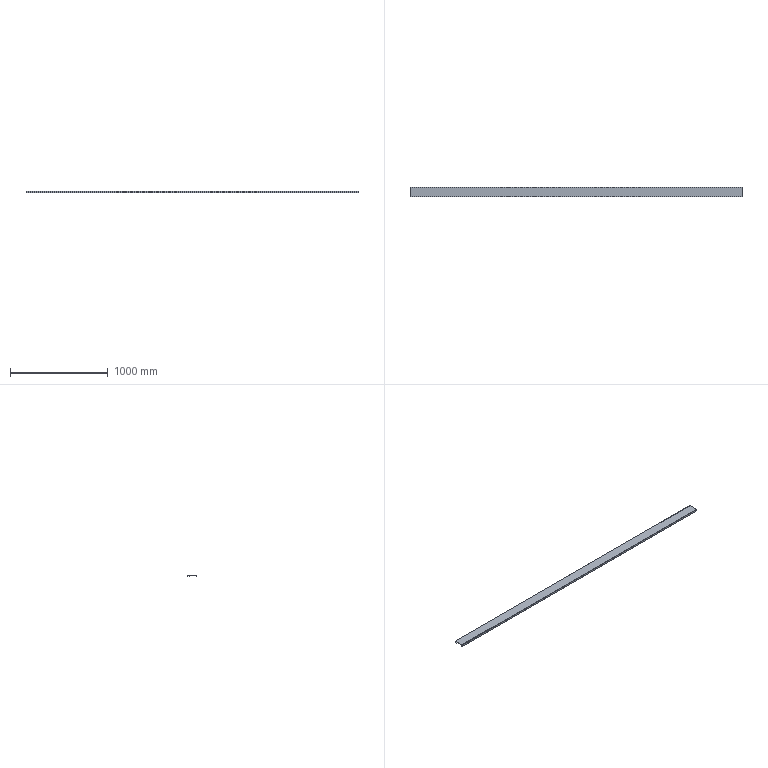Part | STEP file | E3-电柜护栏5踢脚Plate | 1 solid | 18 faces | box 3400 x 100 x 20 mm | volume 781558 mm3 | plane 12 | cylinder 6 | commonest cylinder face diameters 2 x3 5 x3
STEP:
#1=CARTESIAN_POINT('',(0.,0.,0.));
#2=DIRECTION('',(0.,0.,1.));
#3=DIRECTION('',(1.,0.,0.));
#4=AXIS2_PLACEMENT_3D('',#1,#2,#3);
#5=CARTESIAN_POINT('',(-1700.,1.5,-2.5));
#6=VERTEX_POINT('',#5);
#7=CARTESIAN_POINT('',(-1700.,1.5,-20.));
#8=VERTEX_POINT('',#7);
#9=CARTESIAN_POINT('',(-1700.,1.5,-2.5));
#10=DIRECTION('',(0.,0.,-1.));
#11=VECTOR('',#10,1.);
#12=LINE('',#9,#11);
#13=CARTESIAN_POINT('',(1700.,1.5,-2.5));
#14=DIRECTION('',(0.,-1.,0.));
#15=DIRECTION('',(0.,0.,1.));
#16=AXIS2_PLACEMENT_3D('',#13,#14,#15);
#17=PLANE('',#16);
#18=CARTESIAN_POINT('',(0.,3400.));
#19=DIRECTION('',(-1.,0.));
#20=VECTOR('',#19,1.);
#21=LINE('',#18,#20);
#22=(GEOMETRIC_REPRESENTATION_CONTEXT(2)PARAMETRIC_REPRESENTATION_CONTEXT()REPRESENTATION_CONTEXT('',''));
#23=DEFINITIONAL_REPRESENTATION('',(#21),#22);
#24=PCURVE('',#17,#23);
#25=CARTESIAN_POINT('',(-1700.,2.5,-2.5));
#26=DIRECTION('',(-1.,0.,0.));
#27=DIRECTION('',(0.,0.,-1.));
#28=AXIS2_PLACEMENT_3D('',#25,#26,#27);
#29=PLANE('',#28);
#30=CARTESIAN_POINT('',(0.,1.));
#31=DIRECTION('',(1.,0.));
#32=VECTOR('',#31,1.);
#33=LINE('',#30,#32);
#34=(GEOMETRIC_REPRESENTATION_CONTEXT(2)PARAMETRIC_REPRESENTATION_CONTEXT()REPRESENTATION_CONTEXT('',''));
#35=DEFINITIONAL_REPRESENTATION('',(#33),#34);
#36=PCURVE('',#29,#35);
#37=SURFACE_CURVE('',#12,(#24,#36),.PCURVE_S1.);
#38=EDGE_CURVE('',#6,#8,#37,.T.);
#39=ORIENTED_EDGE('',*,*,#38,.F.);
#40=CARTESIAN_POINT('',(1700.,1.5,-2.5));
#41=VERTEX_POINT('',#40);
#42=CARTESIAN_POINT('',(1700.,1.5,-2.5));
#43=DIRECTION('',(-1.,0.,0.));
#44=VECTOR('',#43,1.);
#45=LINE('',#42,#44);
#46=CARTESIAN_POINT('',(0.,0.));
#47=DIRECTION('',(0.,1.));
#48=VECTOR('',#47,1.);
#49=LINE('',#46,#48);
#50=(GEOMETRIC_REPRESENTATION_CONTEXT(2)PARAMETRIC_REPRESENTATION_CONTEXT()REPRESENTATION_CONTEXT('',''));
#51=DEFINITIONAL_REPRESENTATION('',(#49),#50);
#52=PCURVE('',#17,#51);
#53=CARTESIAN_POINT('',(1700.,2.5,-2.5));
#54=DIRECTION('',(-1.,0.,0.));
#55=DIRECTION('',(0.,0.,-1.));
#56=AXIS2_PLACEMENT_3D('',#53,#54,#55);
#57=CYLINDRICAL_SURFACE('',#56,1.);
#58=CARTESIAN_POINT('',(1.571,0.));
#59=DIRECTION('',(0.,1.));
#60=VECTOR('',#59,1.);
#61=LINE('',#58,#60);
#62=(GEOMETRIC_REPRESENTATION_CONTEXT(2)PARAMETRIC_REPRESENTATION_CONTEXT()REPRESENTATION_CONTEXT('',''));
#63=DEFINITIONAL_REPRESENTATION('',(#61),#62);
#64=PCURVE('',#57,#63);
#65=SURFACE_CURVE('',#45,(#52,#64),.PCURVE_S1.);
#66=EDGE_CURVE('',#41,#6,#65,.T.);
#67=ORIENTED_EDGE('',*,*,#66,.F.);
#68=CARTESIAN_POINT('',(1700.,1.5,-20.));
#69=VERTEX_POINT('',#68);
#70=CARTESIAN_POINT('',(1700.,1.5,-2.5));
#71=DIRECTION('',(0.,0.,-1.));
#72=VECTOR('',#71,1.);
#73=LINE('',#70,#72);
#74=CARTESIAN_POINT('',(0.,0.));
#75=DIRECTION('',(-1.,0.));
#76=VECTOR('',#75,1.);
#77=LINE('',#74,#76);
#78=(GEOMETRIC_REPRESENTATION_CONTEXT(2)PARAMETRIC_REPRESENTATION_CONTEXT()REPRESENTATION_CONTEXT('',''));
#79=DEFINITIONAL_REPRESENTATION('',(#77),#78);
#80=PCURVE('',#17,#79);
#81=CARTESIAN_POINT('',(1700.,2.5,-2.5));
#82=DIRECTION('',(-1.,0.,0.));
#83=DIRECTION('',(0.,0.,-1.));
#84=AXIS2_PLACEMENT_3D('',#81,#82,#83);
#85=PLANE('',#84);
#86=CARTESIAN_POINT('',(0.,1.));
#87=DIRECTION('',(1.,0.));
#88=VECTOR('',#87,1.);
#89=LINE('',#86,#88);
#90=(GEOMETRIC_REPRESENTATION_CONTEXT(2)PARAMETRIC_REPRESENTATION_CONTEXT()REPRESENTATION_CONTEXT('',''));
#91=DEFINITIONAL_REPRESENTATION('',(#89),#90);
#92=PCURVE('',#85,#91);
#93=SURFACE_CURVE('',#73,(#80,#92),.PCURVE_S1.);
#94=EDGE_CURVE('',#41,#69,#93,.T.);
#95=ORIENTED_EDGE('',*,*,#94,.T.);
#96=CARTESIAN_POINT('',(1700.,1.5,-20.));
#97=DIRECTION('',(-1.,0.,0.));
#98=VECTOR('',#97,1.);
#99=LINE('',#96,#98);
#100=CARTESIAN_POINT('',(-17.5,0.));
#101=DIRECTION('',(0.,1.));
#102=VECTOR('',#101,1.);
#103=LINE('',#100,#102);
#104=(GEOMETRIC_REPRESENTATION_CONTEXT(2)PARAMETRIC_REPRESENTATION_CONTEXT()REPRESENTATION_CONTEXT('',''));
#105=DEFINITIONAL_REPRESENTATION('',(#103),#104);
#106=PCURVE('',#17,#105);
#107=CARTESIAN_POINT('',(1700.,0.,-20.));
#108=DIRECTION('',(0.,0.,-1.));
#109=DIRECTION('',(1.,0.,0.));
#110=AXIS2_PLACEMENT_3D('',#107,#108,#109);
#111=PLANE('',#110);
#112=CARTESIAN_POINT('',(0.,-1.5));
#113=DIRECTION('',(-1.,0.));
#114=VECTOR('',#113,1.);
#115=LINE('',#112,#114);
#116=(GEOMETRIC_REPRESENTATION_CONTEXT(2)PARAMETRIC_REPRESENTATION_CONTEXT()REPRESENTATION_CONTEXT('',''));
#117=DEFINITIONAL_REPRESENTATION('',(#115),#116);
#118=PCURVE('',#111,#117);
#119=SURFACE_CURVE('',#99,(#106,#118),.PCURVE_S1.);
#120=EDGE_CURVE('',#69,#8,#119,.T.);
#121=ORIENTED_EDGE('',*,*,#120,.T.);
#122=EDGE_LOOP('',(#39,#67,#95,#121));
#123=FACE_BOUND('',#122,.T.);
#124=ADVANCED_FACE('',(#123),#17,.F.);
#125=CARTESIAN_POINT('',(-1700.,0.,-20.));
#126=VERTEX_POINT('',#125);
#127=CARTESIAN_POINT('',(-1700.,0.,-20.));
#128=DIRECTION('',(0.,1.,0.));
#129=VECTOR('',#128,1.);
#130=LINE('',#127,#129);
#131=CARTESIAN_POINT('',(-3400.,0.));
#132=DIRECTION('',(0.,-1.));
#133=VECTOR('',#132,1.);
#134=LINE('',#131,#133);
#135=(GEOMETRIC_REPRESENTATION_CONTEXT(2)PARAMETRIC_REPRESENTATION_CONTEXT()REPRESENTATION_CONTEXT('',''));
#136=DEFINITIONAL_REPRESENTATION('',(#134),#135);
#137=PCURVE('',#111,#136);
#138=CARTESIAN_POINT('',(17.5,2.5));
#139=DIRECTION('',(0.,-1.));
#140=VECTOR('',#139,1.);
#141=LINE('',#138,#140);
#142=(GEOMETRIC_REPRESENTATION_CONTEXT(2)PARAMETRIC_REPRESENTATION_CONTEXT()REPRESENTATION_CONTEXT('',''));
#143=DEFINITIONAL_REPRESENTATION('',(#141),#142);
#144=PCURVE('',#29,#143);
#145=SURFACE_CURVE('',#130,(#137,#144),.PCURVE_S1.);
#146=EDGE_CURVE('',#126,#8,#145,.T.);
#147=ORIENTED_EDGE('',*,*,#146,.T.);
#148=ORIENTED_EDGE('',*,*,#120,.F.);
#149=CARTESIAN_POINT('',(1700.,0.,-20.));
#150=VERTEX_POINT('',#149);
#151=CARTESIAN_POINT('',(1700.,0.,-20.));
#152=DIRECTION('',(0.,1.,0.));
#153=VECTOR('',#152,1.);
#154=LINE('',#151,#153);
#155=CARTESIAN_POINT('',(0.,0.));
#156=DIRECTION('',(0.,-1.));
#157=VECTOR('',#156,1.);
#158=LINE('',#155,#157);
#159=(GEOMETRIC_REPRESENTATION_CONTEXT(2)PARAMETRIC_REPRESENTATION_CONTEXT()REPRESENTATION_CONTEXT('',''));
#160=DEFINITIONAL_REPRESENTATION('',(#158),#159);
#161=PCURVE('',#111,#160);
#162=CARTESIAN_POINT('',(17.5,2.5));
#163=DIRECTION('',(0.,-1.));
#164=VECTOR('',#163,1.);
#165=LINE('',#162,#164);
#166=(GEOMETRIC_REPRESENTATION_CONTEXT(2)PARAMETRIC_REPRESENTATION_CONTEXT()REPRESENTATION_CONTEXT('',''));
#167=DEFINITIONAL_REPRESENTATION('',(#165),#166);
#168=PCURVE('',#85,#167);
#169=SURFACE_CURVE('',#154,(#161,#168),.PCURVE_S1.);
#170=EDGE_CURVE('',#150,#69,#169,.T.);
#171=ORIENTED_EDGE('',*,*,#170,.F.);
#172=CARTESIAN_POINT('',(1700.,0.,-20.));
#173=DIRECTION('',(-1.,0.,0.));
#174=VECTOR('',#173,1.);
#175=LINE('',#172,#174);
#176=CARTESIAN_POINT('',(0.,0.));
#177=DIRECTION('',(-1.,0.));
#178=VECTOR('',#177,1.);
#179=LINE('',#176,#178);
#180=(GEOMETRIC_REPRESENTATION_CONTEXT(2)PARAMETRIC_REPRESENTATION_CONTEXT()REPRESENTATION_CONTEXT('',''));
#181=DEFINITIONAL_REPRESENTATION('',(#179),#180);
#182=PCURVE('',#111,#181);
#183=CARTESIAN_POINT('',(1700.,0.,-2.5));
#184=DIRECTION('',(0.,-1.,0.));
#185=DIRECTION('',(0.,0.,1.));
#186=AXIS2_PLACEMENT_3D('',#183,#184,#185);
#187=PLANE('',#186);
#188=CARTESIAN_POINT('',(-17.5,0.));
#189=DIRECTION('',(0.,1.));
#190=VECTOR('',#189,1.);
#191=LINE('',#188,#190);
#192=(GEOMETRIC_REPRESENTATION_CONTEXT(2)PARAMETRIC_REPRESENTATION_CONTEXT()REPRESENTATION_CONTEXT('',''));
#193=DEFINITIONAL_REPRESENTATION('',(#191),#192);
#194=PCURVE('',#187,#193);
#195=SURFACE_CURVE('',#175,(#182,#194),.PCURVE_S1.);
#196=EDGE_CURVE('',#150,#126,#195,.T.);
#197=ORIENTED_EDGE('',*,*,#196,.T.);
#198=EDGE_LOOP('',(#147,#148,#171,#197));
#199=FACE_BOUND('',#198,.T.);
#200=ADVANCED_FACE('',(#199),#111,.T.);
#201=CARTESIAN_POINT('',(-1700.,0.,-2.5));
#202=VERTEX_POINT('',#201);
#203=CARTESIAN_POINT('',(-1700.,0.,-2.5));
#204=DIRECTION('',(0.,0.,-1.));
#205=VECTOR('',#204,1.);
#206=LINE('',#203,#205);
#207=CARTESIAN_POINT('',(0.,3400.));
#208=DIRECTION('',(-1.,0.));
#209=VECTOR('',#208,1.);
#210=LINE('',#207,#209);
#211=(GEOMETRIC_REPRESENTATION_CONTEXT(2)PARAMETRIC_REPRESENTATION_CONTEXT()REPRESENTATION_CONTEXT('',''));
#212=DEFINITIONAL_REPRESENTATION('',(#210),#211);
#213=PCURVE('',#187,#212);
#214=CARTESIAN_POINT('',(0.,2.5));
#215=DIRECTION('',(1.,0.));
#216=VECTOR('',#215,1.);
#217=LINE('',#214,#216);
#218=(GEOMETRIC_REPRESENTATION_CONTEXT(2)PARAMETRIC_REPRESENTATION_CONTEXT()REPRESENTATION_CONTEXT('',''));
#219=DEFINITIONAL_REPRESENTATION('',(#217),#218);
#220=PCURVE('',#29,#219);
#221=SURFACE_CURVE('',#206,(#213,#220),.PCURVE_S1.);
#222=EDGE_CURVE('',#202,#126,#221,.T.);
#223=ORIENTED_EDGE('',*,*,#222,.T.);
#224=ORIENTED_EDGE('',*,*,#196,.F.);
#225=CARTESIAN_POINT('',(1700.,0.,-2.5));
#226=VERTEX_POINT('',#225);
#227=CARTESIAN_POINT('',(1700.,0.,-2.5));
#228=DIRECTION('',(0.,0.,-1.));
#229=VECTOR('',#228,1.);
#230=LINE('',#227,#229);
#231=CARTESIAN_POINT('',(0.,0.));
#232=DIRECTION('',(-1.,0.));
#233=VECTOR('',#232,1.);
#234=LINE('',#231,#233);
#235=(GEOMETRIC_REPRESENTATION_CONTEXT(2)PARAMETRIC_REPRESENTATION_CONTEXT()REPRESENTATION_CONTEXT('',''));
#236=DEFINITIONAL_REPRESENTATION('',(#234),#235);
#237=PCURVE('',#187,#236);
#238=CARTESIAN_POINT('',(0.,2.5));
#239=DIRECTION('',(1.,0.));
#240=VECTOR('',#239,1.);
#241=LINE('',#238,#240);
#242=(GEOMETRIC_REPRESENTATION_CONTEXT(2)PARAMETRIC_REPRESENTATION_CONTEXT()REPRESENTATION_CONTEXT('',''));
#243=DEFINITIONAL_REPRESENTATION('',(#241),#242);
#244=PCURVE('',#85,#243);
#245=SURFACE_CURVE('',#230,(#237,#244),.PCURVE_S1.);
#246=EDGE_CURVE('',#226,#150,#245,.T.);
#247=ORIENTED_EDGE('',*,*,#246,.F.);
#248=CARTESIAN_POINT('',(1700.,0.,-2.5));
#249=DIRECTION('',(-1.,0.,0.));
#250=VECTOR('',#249,1.);
#251=LINE('',#248,#250);
#252=CARTESIAN_POINT('',(0.,0.));
#253=DIRECTION('',(0.,1.));
#254=VECTOR('',#253,1.);
#255=LINE('',#252,#254);
#256=(GEOMETRIC_REPRESENTATION_CONTEXT(2)PARAMETRIC_REPRESENTATION_CONTEXT()REPRESENTATION_CONTEXT('',''));
#257=DEFINITIONAL_REPRESENTATION('',(#255),#256);
#258=PCURVE('',#187,#257);
#259=CARTESIAN_POINT('',(1700.,2.5,-2.5));
#260=DIRECTION('',(-1.,0.,0.));
#261=DIRECTION('',(0.,0.,-1.));
#262=AXIS2_PLACEMENT_3D('',#259,#260,#261);
#263=CYLINDRICAL_SURFACE('',#262,2.5);
#264=CARTESIAN_POINT('',(1.571,0.));
#265=DIRECTION('',(0.,1.));
#266=VECTOR('',#265,1.);
#267=LINE('',#264,#266);
#268=(GEOMETRIC_REPRESENTATION_CONTEXT(2)PARAMETRIC_REPRESENTATION_CONTEXT()REPRESENTATION_CONTEXT('',''));
#269=DEFINITIONAL_REPRESENTATION('',(#267),#268);
#270=PCURVE('',#263,#269);
#271=SURFACE_CURVE('',#251,(#258,#270),.PCURVE_S1.);
#272=EDGE_CURVE('',#226,#202,#271,.T.);
#273=ORIENTED_EDGE('',*,*,#272,.T.);
#274=EDGE_LOOP('',(#223,#224,#247,#273));
#275=FACE_BOUND('',#274,.T.);
#276=ADVANCED_FACE('',(#275),#187,.T.);
#277=CARTESIAN_POINT('',(-1700.,2.5,0.));
#278=VERTEX_POINT('',#277);
#279=CARTESIAN_POINT('',(-1700.,2.5,-2.5));
#280=DIRECTION('',(1.,0.,0.));
#281=DIRECTION('',(0.,0.,-1.));
#282=AXIS2_PLACEMENT_3D('',#279,#280,#281);
#283=CIRCLE('',#282,2.5);
#284=CARTESIAN_POINT('',(6.283,3400.));
#285=DIRECTION('',(-1.,0.));
#286=VECTOR('',#285,1.);
#287=LINE('',#284,#286);
#288=(GEOMETRIC_REPRESENTATION_CONTEXT(2)PARAMETRIC_REPRESENTATION_CONTEXT()REPRESENTATION_CONTEXT('',''));
#289=DEFINITIONAL_REPRESENTATION('',(#287),#288);
#290=PCURVE('',#263,#289);
#291=CARTESIAN_POINT('',(2.5,0.));
#292=CARTESIAN_POINT('',(2.5,-4.33));
#293=CARTESIAN_POINT('',(-1.25,-2.165));
#294=CARTESIAN_POINT('',(-5.,0.));
#295=CARTESIAN_POINT('',(-1.25,2.165));
#296=CARTESIAN_POINT('',(2.5,4.33));
#297=CARTESIAN_POINT('',(2.5,0.));
#298=(BOUNDED_CURVE()B_SPLINE_CURVE(2,(#291,#292,#293,#294,#295,#296,#297),.UNSPECIFIED.,.T.,.F.)B_SPLINE_CURVE_WITH_KNOTS((1,2,2,2,2,1),(-2.094,0.,2.094,4.189,6.283,8.378),.UNSPECIFIED.)CURVE()GEOMETRIC_REPRESENTATION_ITEM()RATIONAL_B_SPLINE_CURVE((1.,0.5,1.,0.5,1.,0.5,1.))REPRESENTATION_ITEM(''));
#299=(GEOMETRIC_REPRESENTATION_CONTEXT(2)PARAMETRIC_REPRESENTATION_CONTEXT()REPRESENTATION_CONTEXT('',''));
#300=DEFINITIONAL_REPRESENTATION('',(#298),#299);
#301=PCURVE('',#29,#300);
#302=SURFACE_CURVE('',#283,(#290,#301),.PCURVE_S1.);
#303=EDGE_CURVE('',#278,#202,#302,.T.);
#304=ORIENTED_EDGE('',*,*,#303,.T.);
#305=ORIENTED_EDGE('',*,*,#272,.F.);
#306=CARTESIAN_POINT('',(1700.,2.5,0.));
#307=VERTEX_POINT('',#306);
#308=CARTESIAN_POINT('',(1700.,2.5,-2.5));
#309=DIRECTION('',(1.,0.,0.));
#310=DIRECTION('',(0.,0.,-1.));
#311=AXIS2_PLACEMENT_3D('',#308,#309,#310);
#312=CIRCLE('',#311,2.5);
#313=CARTESIAN_POINT('',(6.283,0.));
#314=DIRECTION('',(-1.,0.));
#315=VECTOR('',#314,1.);
#316=LINE('',#313,#315);
#317=(GEOMETRIC_REPRESENTATION_CONTEXT(2)PARAMETRIC_REPRESENTATION_CONTEXT()REPRESENTATION_CONTEXT('',''));
#318=DEFINITIONAL_REPRESENTATION('',(#316),#317);
#319=PCURVE('',#263,#318);
#320=CARTESIAN_POINT('',(2.5,0.));
#321=CARTESIAN_POINT('',(2.5,-4.33));
#322=CARTESIAN_POINT('',(-1.25,-2.165));
#323=CARTESIAN_POINT('',(-5.,0.));
#324=CARTESIAN_POINT('',(-1.25,2.165));
#325=CARTESIAN_POINT('',(2.5,4.33));
#326=CARTESIAN_POINT('',(2.5,0.));
#327=(BOUNDED_CURVE()B_SPLINE_CURVE(2,(#320,#321,#322,#323,#324,#325,#326),.UNSPECIFIED.,.T.,.F.)B_SPLINE_CURVE_WITH_KNOTS((1,2,2,2,2,1),(-2.094,0.,2.094,4.189,6.283,8.378),.UNSPECIFIED.)CURVE()GEOMETRIC_REPRESENTATION_ITEM()RATIONAL_B_SPLINE_CURVE((1.,0.5,1.,0.5,1.,0.5,1.))REPRESENTATION_ITEM(''));
#328=(GEOMETRIC_REPRESENTATION_CONTEXT(2)PARAMETRIC_REPRESENTATION_CONTEXT()REPRESENTATION_CONTEXT('',''));
#329=DEFINITIONAL_REPRESENTATION('',(#327),#328);
#330=PCURVE('',#85,#329);
#331=SURFACE_CURVE('',#312,(#319,#330),.PCURVE_S1.);
#332=EDGE_CURVE('',#307,#226,#331,.T.);
#333=ORIENTED_EDGE('',*,*,#332,.F.);
#334=CARTESIAN_POINT('',(1700.,2.5,0.));
#335=DIRECTION('',(-1.,0.,0.));
#336=VECTOR('',#335,1.);
#337=LINE('',#334,#336);
#338=CARTESIAN_POINT('',(3.142,0.));
#339=DIRECTION('',(0.,1.));
#340=VECTOR('',#339,1.);
#341=LINE('',#338,#340);
#342=(GEOMETRIC_REPRESENTATION_CONTEXT(2)PARAMETRIC_REPRESENTATION_CONTEXT()REPRESENTATION_CONTEXT('',''));
#343=DEFINITIONAL_REPRESENTATION('',(#341),#342);
#344=PCURVE('',#263,#343);
#345=CARTESIAN_POINT('',(1700.,2.5,0.));
#346=DIRECTION('',(0.,0.,1.));
#347=DIRECTION('',(-1.,0.,0.));
#348=AXIS2_PLACEMENT_3D('',#345,#346,#347);
#349=PLANE('',#348);
#350=CARTESIAN_POINT('',(0.,0.));
#351=DIRECTION('',(1.,0.));
#352=VECTOR('',#351,1.);
#353=LINE('',#350,#352);
#354=(GEOMETRIC_REPRESENTATION_CONTEXT(2)PARAMETRIC_REPRESENTATION_CONTEXT()REPRESENTATION_CONTEXT('',''));
#355=DEFINITIONAL_REPRESENTATION('',(#353),#354);
#356=PCURVE('',#349,#355);
#357=SURFACE_CURVE('',#337,(#344,#356),.PCURVE_S1.);
#358=EDGE_CURVE('',#307,#278,#357,.T.);
#359=ORIENTED_EDGE('',*,*,#358,.T.);
#360=EDGE_LOOP('',(#304,#305,#333,#359));
#361=FACE_BOUND('',#360,.T.);
#362=ADVANCED_FACE('',(#361),#263,.T.);
#363=CARTESIAN_POINT('',(-1700.,97.5,0.));
#364=VERTEX_POINT('',#363);
#365=CARTESIAN_POINT('',(-1700.,2.5,0.));
#366=DIRECTION('',(0.,-1.,0.));
#367=VECTOR('',#366,1.);
#368=LINE('',#365,#367);
#369=CARTESIAN_POINT('',(3400.,0.));
#370=DIRECTION('',(0.,1.));
#371=VECTOR('',#370,1.);
#372=LINE('',#369,#371);
#373=(GEOMETRIC_REPRESENTATION_CONTEXT(2)PARAMETRIC_REPRESENTATION_CONTEXT()REPRESENTATION_CONTEXT('',''));
#374=DEFINITIONAL_REPRESENTATION('',(#372),#373);
#375=PCURVE('',#349,#374);
#376=CARTESIAN_POINT('',(-2.5,0.));
#377=DIRECTION('',(0.,1.));
#378=VECTOR('',#377,1.);
#379=LINE('',#376,#378);
#380=(GEOMETRIC_REPRESENTATION_CONTEXT(2)PARAMETRIC_REPRESENTATION_CONTEXT()REPRESENTATION_CONTEXT('',''));
#381=DEFINITIONAL_REPRESENTATION('',(#379),#380);
#382=PCURVE('',#29,#381);
#383=SURFACE_CURVE('',#368,(#375,#382),.PCURVE_S1.);
#384=EDGE_CURVE('',#364,#278,#383,.T.);
#385=ORIENTED_EDGE('',*,*,#384,.T.);
#386=ORIENTED_EDGE('',*,*,#358,.F.);
#387=CARTESIAN_POINT('',(1700.,97.5,0.));
#388=VERTEX_POINT('',#387);
#389=CARTESIAN_POINT('',(1700.,2.5,0.));
#390=DIRECTION('',(0.,-1.,0.));
#391=VECTOR('',#390,1.);
#392=LINE('',#389,#391);
#393=CARTESIAN_POINT('',(0.,0.));
#394=DIRECTION('',(0.,1.));
#395=VECTOR('',#394,1.);
#396=LINE('',#393,#395);
#397=(GEOMETRIC_REPRESENTATION_CONTEXT(2)PARAMETRIC_REPRESENTATION_CONTEXT()REPRESENTATION_CONTEXT('',''));
#398=DEFINITIONAL_REPRESENTATION('',(#396),#397);
#399=PCURVE('',#349,#398);
#400=CARTESIAN_POINT('',(-2.5,0.));
#401=DIRECTION('',(0.,1.));
#402=VECTOR('',#401,1.);
#403=LINE('',#400,#402);
#404=(GEOMETRIC_REPRESENTATION_CONTEXT(2)PARAMETRIC_REPRESENTATION_CONTEXT()REPRESENTATION_CONTEXT('',''));
#405=DEFINITIONAL_REPRESENTATION('',(#403),#404);
#406=PCURVE('',#85,#405);
#407=SURFACE_CURVE('',#392,(#399,#406),.PCURVE_S1.);
#408=EDGE_CURVE('',#388,#307,#407,.T.);
#409=ORIENTED_EDGE('',*,*,#408,.F.);
#410=CARTESIAN_POINT('',(1700.,97.5,0.));
#411=DIRECTION('',(-1.,0.,0.));
#412=VECTOR('',#411,1.);
#413=LINE('',#410,#412);
#414=CARTESIAN_POINT('',(0.,-95.));
#415=DIRECTION('',(1.,0.));
#416=VECTOR('',#415,1.);
#417=LINE('',#414,#416);
#418=(GEOMETRIC_REPRESENTATION_CONTEXT(2)PARAMETRIC_REPRESENTATION_CONTEXT()REPRESENTATION_CONTEXT('',''));
#419=DEFINITIONAL_REPRESENTATION('',(#417),#418);
#420=PCURVE('',#349,#419);
#421=CARTESIAN_POINT('',(1700.,97.5,-2.5));
#422=DIRECTION('',(-1.,0.,0.));
#423=DIRECTION('',(0.,0.,-1.));
#424=AXIS2_PLACEMENT_3D('',#421,#422,#423);
#425=CYLINDRICAL_SURFACE('',#424,2.5);
#426=CARTESIAN_POINT('',(3.142,0.));
#427=DIRECTION('',(0.,1.));
#428=VECTOR('',#427,1.);
#429=LINE('',#426,#428);
#430=(GEOMETRIC_REPRESENTATION_CONTEXT(2)PARAMETRIC_REPRESENTATION_CONTEXT()REPRESENTATION_CONTEXT('',''));
#431=DEFINITIONAL_REPRESENTATION('',(#429),#430);
#432=PCURVE('',#425,#431);
#433=SURFACE_CURVE('',#413,(#420,#432),.PCURVE_S1.);
#434=EDGE_CURVE('',#388,#364,#433,.T.);
#435=ORIENTED_EDGE('',*,*,#434,.T.);
#436=EDGE_LOOP('',(#385,#386,#409,#435));
#437=FACE_BOUND('',#436,.T.);
#438=ADVANCED_FACE('',(#437),#349,.T.);
#439=CARTESIAN_POINT('',(-1700.,100.,-2.5));
#440=VERTEX_POINT('',#439);
#441=CARTESIAN_POINT('',(-1700.,97.5,-2.5));
#442=DIRECTION('',(1.,0.,0.));
#443=DIRECTION('',(0.,0.,1.));
#444=AXIS2_PLACEMENT_3D('',#441,#442,#443);
#445=CIRCLE('',#444,2.5);
#446=CARTESIAN_POINT('',(9.425,3400.));
#447=DIRECTION('',(-1.,0.));
#448=VECTOR('',#447,1.);
#449=LINE('',#446,#448);
#450=(GEOMETRIC_REPRESENTATION_CONTEXT(2)PARAMETRIC_REPRESENTATION_CONTEXT()REPRESENTATION_CONTEXT('',''));
#451=DEFINITIONAL_REPRESENTATION('',(#449),#450);
#452=PCURVE('',#425,#451);
#453=CARTESIAN_POINT('',(-2.5,-95.));
#454=CARTESIAN_POINT('',(-2.5,-90.67));
#455=CARTESIAN_POINT('',(1.25,-92.835));
#456=CARTESIAN_POINT('',(5.,-95.));
#457=CARTESIAN_POINT('',(1.25,-97.165));
#458=CARTESIAN_POINT('',(-2.5,-99.33));
#459=CARTESIAN_POINT('',(-2.5,-95.));
#460=(BOUNDED_CURVE()B_SPLINE_CURVE(2,(#453,#454,#455,#456,#457,#458,#459),.UNSPECIFIED.,.T.,.F.)B_SPLINE_CURVE_WITH_KNOTS((1,2,2,2,2,1),(-2.094,0.,2.094,4.189,6.283,8.378),.UNSPECIFIED.)CURVE()GEOMETRIC_REPRESENTATION_ITEM()RATIONAL_B_SPLINE_CURVE((1.,0.5,1.,0.5,1.,0.5,1.))REPRESENTATION_ITEM(''));
#461=(GEOMETRIC_REPRESENTATION_CONTEXT(2)PARAMETRIC_REPRESENTATION_CONTEXT()REPRESENTATION_CONTEXT('',''));
#462=DEFINITIONAL_REPRESENTATION('',(#460),#461);
#463=PCURVE('',#29,#462);
#464=SURFACE_CURVE('',#445,(#452,#463),.PCURVE_S1.);
#465=EDGE_CURVE('',#440,#364,#464,.T.);
#466=ORIENTED_EDGE('',*,*,#465,.T.);
#467=ORIENTED_EDGE('',*,*,#434,.F.);
#468=CARTESIAN_POINT('',(1700.,100.,-2.5));
#469=VERTEX_POINT('',#468);
#470=CARTESIAN_POINT('',(1700.,97.5,-2.5));
#471=DIRECTION('',(1.,0.,0.));
#472=DIRECTION('',(0.,0.,1.));
#473=AXIS2_PLACEMENT_3D('',#470,#471,#472);
#474=CIRCLE('',#473,2.5);
#475=CARTESIAN_POINT('',(9.425,0.));
#476=DIRECTION('',(-1.,0.));
#477=VECTOR('',#476,1.);
#478=LINE('',#475,#477);
#479=(GEOMETRIC_REPRESENTATION_CONTEXT(2)PARAMETRIC_REPRESENTATION_CONTEXT()REPRESENTATION_CONTEXT('',''));
#480=DEFINITIONAL_REPRESENTATION('',(#478),#479);
#481=PCURVE('',#425,#480);
#482=CARTESIAN_POINT('',(-2.5,-95.));
#483=CARTESIAN_POINT('',(-2.5,-90.67));
#484=CARTESIAN_POINT('',(1.25,-92.835));
#485=CARTESIAN_POINT('',(5.,-95.));
#486=CARTESIAN_POINT('',(1.25,-97.165));
#487=CARTESIAN_POINT('',(-2.5,-99.33));
#488=CARTESIAN_POINT('',(-2.5,-95.));
#489=(BOUNDED_CURVE()B_SPLINE_CURVE(2,(#482,#483,#484,#485,#486,#487,#488),.UNSPECIFIED.,.T.,.F.)B_SPLINE_CURVE_WITH_KNOTS((1,2,2,2,2,1),(-2.094,0.,2.094,4.189,6.283,8.378),.UNSPECIFIED.)CURVE()GEOMETRIC_REPRESENTATION_ITEM()RATIONAL_B_SPLINE_CURVE((1.,0.5,1.,0.5,1.,0.5,1.))REPRESENTATION_ITEM(''));
#490=(GEOMETRIC_REPRESENTATION_CONTEXT(2)PARAMETRIC_REPRESENTATION_CONTEXT()REPRESENTATION_CONTEXT('',''));
#491=DEFINITIONAL_REPRESENTATION('',(#489),#490);
#492=PCURVE('',#85,#491);
#493=SURFACE_CURVE('',#474,(#481,#492),.PCURVE_S1.);
#494=EDGE_CURVE('',#469,#388,#493,.T.);
#495=ORIENTED_EDGE('',*,*,#494,.F.);
#496=CARTESIAN_POINT('',(1700.,100.,-2.5));
#497=DIRECTION('',(-1.,0.,0.));
#498=VECTOR('',#497,1.);
#499=LINE('',#496,#498);
#500=CARTESIAN_POINT('',(4.712,0.));
#501=DIRECTION('',(0.,1.));
#502=VECTOR('',#501,1.);
#503=LINE('',#500,#502);
#504=(GEOMETRIC_REPRESENTATION_CONTEXT(2)PARAMETRIC_REPRESENTATION_CONTEXT()REPRESENTATION_CONTEXT('',''));
#505=DEFINITIONAL_REPRESENTATION('',(#503),#504);
#506=PCURVE('',#425,#505);
#507=CARTESIAN_POINT('',(1700.,100.,-2.5));
#508=DIRECTION('',(0.,1.,0.));
#509=DIRECTION('',(0.,0.,-1.));
#510=AXIS2_PLACEMENT_3D('',#507,#508,#509);
#511=PLANE('',#510);
#512=CARTESIAN_POINT('',(0.,0.));
#513=DIRECTION('',(0.,1.));
#514=VECTOR('',#513,1.);
#515=LINE('',#512,#514);
#516=(GEOMETRIC_REPRESENTATION_CONTEXT(2)PARAMETRIC_REPRESENTATION_CONTEXT()REPRESENTATION_CONTEXT('',''));
#517=DEFINITIONAL_REPRESENTATION('',(#515),#516);
#518=PCURVE('',#511,#517);
#519=SURFACE_CURVE('',#499,(#506,#518),.PCURVE_S1.);
#520=EDGE_CURVE('',#469,#440,#519,.T.);
#521=ORIENTED_EDGE('',*,*,#520,.T.);
#522=EDGE_LOOP('',(#466,#467,#495,#521));
#523=FACE_BOUND('',#522,.T.);
#524=ADVANCED_FACE('',(#523),#425,.T.);
#525=CARTESIAN_POINT('',(-1700.,100.,-17.5));
#526=VERTEX_POINT('',#525);
#527=CARTESIAN_POINT('',(-1700.,100.,-2.5));
#528=DIRECTION('',(0.,0.,1.));
#529=VECTOR('',#528,1.);
#530=LINE('',#527,#529);
#531=CARTESIAN_POINT('',(0.,3400.));
#532=DIRECTION('',(-1.,0.));
#533=VECTOR('',#532,1.);
#534=LINE('',#531,#533);
#535=(GEOMETRIC_REPRESENTATION_CONTEXT(2)PARAMETRIC_REPRESENTATION_CONTEXT()REPRESENTATION_CONTEXT('',''));
#536=DEFINITIONAL_REPRESENTATION('',(#534),#535);
#537=PCURVE('',#511,#536);
#538=CARTESIAN_POINT('',(0.,-97.5));
#539=DIRECTION('',(-1.,0.));
#540=VECTOR('',#539,1.);
#541=LINE('',#538,#540);
#542=(GEOMETRIC_REPRESENTATION_CONTEXT(2)PARAMETRIC_REPRESENTATION_CONTEXT()REPRESENTATION_CONTEXT('',''));
#543=DEFINITIONAL_REPRESENTATION('',(#541),#542);
#544=PCURVE('',#29,#543);
#545=SURFACE_CURVE('',#530,(#537,#544),.PCURVE_S1.);
#546=EDGE_CURVE('',#526,#440,#545,.T.);
#547=ORIENTED_EDGE('',*,*,#546,.T.);
#548=ORIENTED_EDGE('',*,*,#520,.F.);
#549=CARTESIAN_POINT('',(1700.,100.,-17.5));
#550=VERTEX_POINT('',#549);
#551=CARTESIAN_POINT('',(1700.,100.,-2.5));
#552=DIRECTION('',(0.,0.,1.));
#553=VECTOR('',#552,1.);
#554=LINE('',#551,#553);
#555=CARTESIAN_POINT('',(0.,0.));
#556=DIRECTION('',(-1.,0.));
#557=VECTOR('',#556,1.);
#558=LINE('',#555,#557);
#559=(GEOMETRIC_REPRESENTATION_CONTEXT(2)PARAMETRIC_REPRESENTATION_CONTEXT()REPRESENTATION_CONTEXT('',''));
#560=DEFINITIONAL_REPRESENTATION('',(#558),#559);
#561=PCURVE('',#511,#560);
#562=CARTESIAN_POINT('',(0.,-97.5));
#563=DIRECTION('',(-1.,0.));
#564=VECTOR('',#563,1.);
#565=LINE('',#562,#564);
#566=(GEOMETRIC_REPRESENTATION_CONTEXT(2)PARAMETRIC_REPRESENTATION_CONTEXT()REPRESENTATION_CONTEXT('',''));
#567=DEFINITIONAL_REPRESENTATION('',(#565),#566);
#568=PCURVE('',#85,#567);
#569=SURFACE_CURVE('',#554,(#561,#568),.PCURVE_S1.);
#570=EDGE_CURVE('',#550,#469,#569,.T.);
#571=ORIENTED_EDGE('',*,*,#570,.F.);
#572=CARTESIAN_POINT('',(1700.,100.,-17.5));
#573=DIRECTION('',(-1.,0.,0.));
#574=VECTOR('',#573,1.);
#575=LINE('',#572,#574);
#576=CARTESIAN_POINT('',(15.,0.));
#577=DIRECTION('',(0.,1.));
#578=VECTOR('',#577,1.);
#579=LINE('',#576,#578);
#580=(GEOMETRIC_REPRESENTATION_CONTEXT(2)PARAMETRIC_REPRESENTATION_CONTEXT()REPRESENTATION_CONTEXT('',''));
#581=DEFINITIONAL_REPRESENTATION('',(#579),#580);
#582=PCURVE('',#511,#581);
#583=CARTESIAN_POINT('',(1700.,97.5,-17.5));
#584=DIRECTION('',(-1.,0.,0.));
#585=DIRECTION('',(0.,0.,-1.));
#586=AXIS2_PLACEMENT_3D('',#583,#584,#585);
#587=CYLINDRICAL_SURFACE('',#586,2.5);
#588=CARTESIAN_POINT('',(4.712,0.));
#589=DIRECTION('',(0.,1.));
#590=VECTOR('',#589,1.);
#591=LINE('',#588,#590);
#592=(GEOMETRIC_REPRESENTATION_CONTEXT(2)PARAMETRIC_REPRESENTATION_CONTEXT()REPRESENTATION_CONTEXT('',''));
#593=DEFINITIONAL_REPRESENTATION('',(#591),#592);
#594=PCURVE('',#587,#593);
#595=SURFACE_CURVE('',#575,(#582,#594),.PCURVE_S1.);
#596=EDGE_CURVE('',#550,#526,#595,.T.);
#597=ORIENTED_EDGE('',*,*,#596,.T.);
#598=EDGE_LOOP('',(#547,#548,#571,#597));
#599=FACE_BOUND('',#598,.T.);
#600=ADVANCED_FACE('',(#599),#511,.T.);
#601=CARTESIAN_POINT('',(-1700.,97.5,-20.));
#602=VERTEX_POINT('',#601);
#603=CARTESIAN_POINT('',(-1700.,97.5,-17.5));
#604=DIRECTION('',(1.,0.,0.));
#605=DIRECTION('',(0.,0.,1.));
#606=AXIS2_PLACEMENT_3D('',#603,#604,#605);
#607=CIRCLE('',#606,2.5);
#608=CARTESIAN_POINT('',(9.425,3400.));
#609=DIRECTION('',(-1.,0.));
#610=VECTOR('',#609,1.);
#611=LINE('',#608,#610);
#612=(GEOMETRIC_REPRESENTATION_CONTEXT(2)PARAMETRIC_REPRESENTATION_CONTEXT()REPRESENTATION_CONTEXT('',''));
#613=DEFINITIONAL_REPRESENTATION('',(#611),#612);
#614=PCURVE('',#587,#613);
#615=CARTESIAN_POINT('',(12.5,-95.));
#616=CARTESIAN_POINT('',(12.5,-90.67));
#617=CARTESIAN_POINT('',(16.25,-92.835));
#618=CARTESIAN_POINT('',(20.,-95.));
#619=CARTESIAN_POINT('',(16.25,-97.165));
#620=CARTESIAN_POINT('',(12.5,-99.33));
#621=CARTESIAN_POINT('',(12.5,-95.));
#622=(BOUNDED_CURVE()B_SPLINE_CURVE(2,(#615,#616,#617,#618,#619,#620,#621),.UNSPECIFIED.,.T.,.F.)B_SPLINE_CURVE_WITH_KNOTS((1,2,2,2,2,1),(-2.094,0.,2.094,4.189,6.283,8.378),.UNSPECIFIED.)CURVE()GEOMETRIC_REPRESENTATION_ITEM()RATIONAL_B_SPLINE_CURVE((1.,0.5,1.,0.5,1.,0.5,1.))REPRESENTATION_ITEM(''));
#623=(GEOMETRIC_REPRESENTATION_CONTEXT(2)PARAMETRIC_REPRESENTATION_CONTEXT()REPRESENTATION_CONTEXT('',''));
#624=DEFINITIONAL_REPRESENTATION('',(#622),#623);
#625=PCURVE('',#29,#624);
#626=SURFACE_CURVE('',#607,(#614,#625),.PCURVE_S1.);
#627=EDGE_CURVE('',#602,#526,#626,.T.);
#628=ORIENTED_EDGE('',*,*,#627,.T.);
#629=ORIENTED_EDGE('',*,*,#596,.F.);
#630=CARTESIAN_POINT('',(1700.,97.5,-20.));
#631=VERTEX_POINT('',#630);
#632=CARTESIAN_POINT('',(1700.,97.5,-17.5));
#633=DIRECTION('',(1.,0.,0.));
#634=DIRECTION('',(0.,0.,1.));
#635=AXIS2_PLACEMENT_3D('',#632,#633,#634);
#636=CIRCLE('',#635,2.5);
#637=CARTESIAN_POINT('',(9.425,0.));
#638=DIRECTION('',(-1.,0.));
#639=VECTOR('',#638,1.);
#640=LINE('',#637,#639);
#641=(GEOMETRIC_REPRESENTATION_CONTEXT(2)PARAMETRIC_REPRESENTATION_CONTEXT()REPRESENTATION_CONTEXT('',''));
#642=DEFINITIONAL_REPRESENTATION('',(#640),#641);
#643=PCURVE('',#587,#642);
#644=CARTESIAN_POINT('',(12.5,-95.));
#645=CARTESIAN_POINT('',(12.5,-90.67));
#646=CARTESIAN_POINT('',(16.25,-92.835));
#647=CARTESIAN_POINT('',(20.,-95.));
#648=CARTESIAN_POINT('',(16.25,-97.165));
#649=CARTESIAN_POINT('',(12.5,-99.33));
#650=CARTESIAN_POINT('',(12.5,-95.));
#651=(BOUNDED_CURVE()B_SPLINE_CURVE(2,(#644,#645,#646,#647,#648,#649,#650),.UNSPECIFIED.,.T.,.F.)B_SPLINE_CURVE_WITH_KNOTS((1,2,2,2,2,1),(-2.094,0.,2.094,4.189,6.283,8.378),.UNSPECIFIED.)CURVE()GEOMETRIC_REPRESENTATION_ITEM()RATIONAL_B_SPLINE_CURVE((1.,0.5,1.,0.5,1.,0.5,1.))REPRESENTATION_ITEM(''));
#652=(GEOMETRIC_REPRESENTATION_CONTEXT(2)PARAMETRIC_REPRESENTATION_CONTEXT()REPRESENTATION_CONTEXT('',''));
#653=DEFINITIONAL_REPRESENTATION('',(#651),#652);
#654=PCURVE('',#85,#653);
#655=SURFACE_CURVE('',#636,(#643,#654),.PCURVE_S1.);
#656=EDGE_CURVE('',#631,#550,#655,.T.);
#657=ORIENTED_EDGE('',*,*,#656,.F.);
#658=CARTESIAN_POINT('',(1700.,97.5,-20.));
#659=DIRECTION('',(-1.,0.,0.));
#660=VECTOR('',#659,1.);
#661=LINE('',#658,#660);
#662=CARTESIAN_POINT('',(6.283,0.));
#663=DIRECTION('',(0.,1.));
#664=VECTOR('',#663,1.);
#665=LINE('',#662,#664);
#666=(GEOMETRIC_REPRESENTATION_CONTEXT(2)PARAMETRIC_REPRESENTATION_CONTEXT()REPRESENTATION_CONTEXT('',''));
#667=DEFINITIONAL_REPRESENTATION('',(#665),#666);
#668=PCURVE('',#587,#667);
#669=CARTESIAN_POINT('',(1700.,97.5,-20.));
#670=DIRECTION('',(0.,0.,-1.));
#671=DIRECTION('',(1.,0.,0.));
#672=AXIS2_PLACEMENT_3D('',#669,#670,#671);
#673=PLANE('',#672);
#674=CARTESIAN_POINT('',(0.,0.));
#675=DIRECTION('',(-1.,0.));
#676=VECTOR('',#675,1.);
#677=LINE('',#674,#676);
#678=(GEOMETRIC_REPRESENTATION_CONTEXT(2)PARAMETRIC_REPRESENTATION_CONTEXT()REPRESENTATION_CONTEXT('',''));
#679=DEFINITIONAL_REPRESENTATION('',(#677),#678);
#680=PCURVE('',#673,#679);
#681=SURFACE_CURVE('',#661,(#668,#680),.PCURVE_S1.);
#682=EDGE_CURVE('',#631,#602,#681,.T.);
#683=ORIENTED_EDGE('',*,*,#682,.T.);
#684=EDGE_LOOP('',(#628,#629,#657,#683));
#685=FACE_BOUND('',#684,.T.);
#686=ADVANCED_FACE('',(#685),#587,.T.);
#687=CARTESIAN_POINT('',(-1700.,80.,-20.));
#688=VERTEX_POINT('',#687);
#689=CARTESIAN_POINT('',(-1700.,97.5,-20.));
#690=DIRECTION('',(0.,1.,0.));
#691=VECTOR('',#690,1.);
#692=LINE('',#689,#691);
#693=CARTESIAN_POINT('',(-3400.,0.));
#694=DIRECTION('',(0.,-1.));
#695=VECTOR('',#694,1.);
#696=LINE('',#693,#695);
#697=(GEOMETRIC_REPRESENTATION_CONTEXT(2)PARAMETRIC_REPRESENTATION_CONTEXT()REPRESENTATION_CONTEXT('',''));
#698=DEFINITIONAL_REPRESENTATION('',(#696),#697);
#699=PCURVE('',#673,#698);
#700=CARTESIAN_POINT('',(17.5,-95.));
#701=DIRECTION('',(0.,-1.));
#702=VECTOR('',#701,1.);
#703=LINE('',#700,#702);
#704=(GEOMETRIC_REPRESENTATION_CONTEXT(2)PARAMETRIC_REPRESENTATION_CONTEXT()REPRESENTATION_CONTEXT('',''));
#705=DEFINITIONAL_REPRESENTATION('',(#703),#704);
#706=PCURVE('',#29,#705);
#707=SURFACE_CURVE('',#692,(#699,#706),.PCURVE_S1.);
#708=EDGE_CURVE('',#688,#602,#707,.T.);
#709=ORIENTED_EDGE('',*,*,#708,.T.);
#710=ORIENTED_EDGE('',*,*,#682,.F.);
#711=CARTESIAN_POINT('',(1700.,80.,-20.));
#712=VERTEX_POINT('',#711);
#713=CARTESIAN_POINT('',(1700.,97.5,-20.));
#714=DIRECTION('',(0.,1.,0.));
#715=VECTOR('',#714,1.);
#716=LINE('',#713,#715);
#717=CARTESIAN_POINT('',(0.,0.));
#718=DIRECTION('',(0.,-1.));
#719=VECTOR('',#718,1.);
#720=LINE('',#717,#719);
#721=(GEOMETRIC_REPRESENTATION_CONTEXT(2)PARAMETRIC_REPRESENTATION_CONTEXT()REPRESENTATION_CONTEXT('',''));
#722=DEFINITIONAL_REPRESENTATION('',(#720),#721);
#723=PCURVE('',#673,#722);
#724=CARTESIAN_POINT('',(17.5,-95.));
#725=DIRECTION('',(0.,-1.));
#726=VECTOR('',#725,1.);
#727=LINE('',#724,#726);
#728=(GEOMETRIC_REPRESENTATION_CONTEXT(2)PARAMETRIC_REPRESENTATION_CONTEXT()REPRESENTATION_CONTEXT('',''));
#729=DEFINITIONAL_REPRESENTATION('',(#727),#728);
#730=PCURVE('',#85,#729);
#731=SURFACE_CURVE('',#716,(#723,#730),.PCURVE_S1.);
#732=EDGE_CURVE('',#712,#631,#731,.T.);
#733=ORIENTED_EDGE('',*,*,#732,.F.);
#734=CARTESIAN_POINT('',(1700.,80.,-20.));
#735=DIRECTION('',(-1.,0.,0.));
#736=VECTOR('',#735,1.);
#737=LINE('',#734,#736);
#738=CARTESIAN_POINT('',(0.,17.5));
#739=DIRECTION('',(-1.,0.));
#740=VECTOR('',#739,1.);
#741=LINE('',#738,#740);
#742=(GEOMETRIC_REPRESENTATION_CONTEXT(2)PARAMETRIC_REPRESENTATION_CONTEXT()REPRESENTATION_CONTEXT('',''));
#743=DEFINITIONAL_REPRESENTATION('',(#741),#742);
#744=PCURVE('',#673,#743);
#745=CARTESIAN_POINT('',(1700.,80.,-18.5));
#746=DIRECTION('',(0.,-1.,0.));
#747=DIRECTION('',(0.,0.,1.));
#748=AXIS2_PLACEMENT_3D('',#745,#746,#747);
#749=PLANE('',#748);
#750=CARTESIAN_POINT('',(-1.5,0.));
#751=DIRECTION('',(0.,1.));
#752=VECTOR('',#751,1.);
#753=LINE('',#750,#752);
#754=(GEOMETRIC_REPRESENTATION_CONTEXT(2)PARAMETRIC_REPRESENTATION_CONTEXT()REPRESENTATION_CONTEXT('',''));
#755=DEFINITIONAL_REPRESENTATION('',(#753),#754);
#756=PCURVE('',#749,#755);
#757=SURFACE_CURVE('',#737,(#744,#756),.PCURVE_S1.);
#758=EDGE_CURVE('',#712,#688,#757,.T.);
#759=ORIENTED_EDGE('',*,*,#758,.T.);
#760=EDGE_LOOP('',(#709,#710,#733,#759));
#761=FACE_BOUND('',#760,.T.);
#762=ADVANCED_FACE('',(#761),#673,.T.);
#763=CARTESIAN_POINT('',(-1700.,80.,-18.5));
#764=VERTEX_POINT('',#763);
#765=CARTESIAN_POINT('',(-1700.,80.,-18.5));
#766=DIRECTION('',(0.,0.,-1.));
#767=VECTOR('',#766,1.);
#768=LINE('',#765,#767);
#769=CARTESIAN_POINT('',(0.,3400.));
#770=DIRECTION('',(-1.,0.));
#771=VECTOR('',#770,1.);
#772=LINE('',#769,#771);
#773=(GEOMETRIC_REPRESENTATION_CONTEXT(2)PARAMETRIC_REPRESENTATION_CONTEXT()REPRESENTATION_CONTEXT('',''));
#774=DEFINITIONAL_REPRESENTATION('',(#772),#773);
#775=PCURVE('',#749,#774);
#776=CARTESIAN_POINT('',(16.,-77.5));
#777=DIRECTION('',(1.,0.));
#778=VECTOR('',#777,1.);
#779=LINE('',#776,#778);
#780=(GEOMETRIC_REPRESENTATION_CONTEXT(2)PARAMETRIC_REPRESENTATION_CONTEXT()REPRESENTATION_CONTEXT('',''));
#781=DEFINITIONAL_REPRESENTATION('',(#779),#780);
#782=PCURVE('',#29,#781);
#783=SURFACE_CURVE('',#768,(#775,#782),.PCURVE_S1.);
#784=EDGE_CURVE('',#764,#688,#783,.T.);
#785=ORIENTED_EDGE('',*,*,#784,.T.);
#786=ORIENTED_EDGE('',*,*,#758,.F.);
#787=CARTESIAN_POINT('',(1700.,80.,-18.5));
#788=VERTEX_POINT('',#787);
#789=CARTESIAN_POINT('',(1700.,80.,-18.5));
#790=DIRECTION('',(0.,0.,-1.));
#791=VECTOR('',#790,1.);
#792=LINE('',#789,#791);
#793=CARTESIAN_POINT('',(0.,0.));
#794=DIRECTION('',(-1.,0.));
#795=VECTOR('',#794,1.);
#796=LINE('',#793,#795);
#797=(GEOMETRIC_REPRESENTATION_CONTEXT(2)PARAMETRIC_REPRESENTATION_CONTEXT()REPRESENTATION_CONTEXT('',''));
#798=DEFINITIONAL_REPRESENTATION('',(#796),#797);
#799=PCURVE('',#749,#798);
#800=CARTESIAN_POINT('',(16.,-77.5));
#801=DIRECTION('',(1.,0.));
#802=VECTOR('',#801,1.);
#803=LINE('',#800,#802);
#804=(GEOMETRIC_REPRESENTATION_CONTEXT(2)PARAMETRIC_REPRESENTATION_CONTEXT()REPRESENTATION_CONTEXT('',''));
#805=DEFINITIONAL_REPRESENTATION('',(#803),#804);
#806=PCURVE('',#85,#805);
#807=SURFACE_CURVE('',#792,(#799,#806),.PCURVE_S1.);
#808=EDGE_CURVE('',#788,#712,#807,.T.);
#809=ORIENTED_EDGE('',*,*,#808,.F.);
#810=CARTESIAN_POINT('',(1700.,80.,-18.5));
#811=DIRECTION('',(-1.,0.,0.));
#812=VECTOR('',#811,1.);
#813=LINE('',#810,#812);
#814=CARTESIAN_POINT('',(0.,0.));
#815=DIRECTION('',(0.,1.));
#816=VECTOR('',#815,1.);
#817=LINE('',#814,#816);
#818=(GEOMETRIC_REPRESENTATION_CONTEXT(2)PARAMETRIC_REPRESENTATION_CONTEXT()REPRESENTATION_CONTEXT('',''));
#819=DEFINITIONAL_REPRESENTATION('',(#817),#818);
#820=PCURVE('',#749,#819);
#821=CARTESIAN_POINT('',(1700.,97.5,-18.5));
#822=DIRECTION('',(0.,0.,-1.));
#823=DIRECTION('',(1.,0.,0.));
#824=AXIS2_PLACEMENT_3D('',#821,#822,#823);
#825=PLANE('',#824);
#826=CARTESIAN_POINT('',(0.,17.5));
#827=DIRECTION('',(-1.,0.));
#828=VECTOR('',#827,1.);
#829=LINE('',#826,#828);
#830=(GEOMETRIC_REPRESENTATION_CONTEXT(2)PARAMETRIC_REPRESENTATION_CONTEXT()REPRESENTATION_CONTEXT('',''));
#831=DEFINITIONAL_REPRESENTATION('',(#829),#830);
#832=PCURVE('',#825,#831);
#833=SURFACE_CURVE('',#813,(#820,#832),.PCURVE_S1.);
#834=EDGE_CURVE('',#788,#764,#833,.T.);
#835=ORIENTED_EDGE('',*,*,#834,.T.);
#836=EDGE_LOOP('',(#785,#786,#809,#835));
#837=FACE_BOUND('',#836,.T.);
#838=ADVANCED_FACE('',(#837),#749,.T.);
#839=CARTESIAN_POINT('',(-1700.,97.5,-18.5));
#840=VERTEX_POINT('',#839);
#841=CARTESIAN_POINT('',(-1700.,97.5,-18.5));
#842=DIRECTION('',(0.,1.,0.));
#843=VECTOR('',#842,1.);
#844=LINE('',#841,#843);
#845=CARTESIAN_POINT('',(-3400.,0.));
#846=DIRECTION('',(0.,-1.));
#847=VECTOR('',#846,1.);
#848=LINE('',#845,#847);
#849=(GEOMETRIC_REPRESENTATION_CONTEXT(2)PARAMETRIC_REPRESENTATION_CONTEXT()REPRESENTATION_CONTEXT('',''));
#850=DEFINITIONAL_REPRESENTATION('',(#848),#849);
#851=PCURVE('',#825,#850);
#852=CARTESIAN_POINT('',(16.,-95.));
#853=DIRECTION('',(0.,-1.));
#854=VECTOR('',#853,1.);
#855=LINE('',#852,#854);
#856=(GEOMETRIC_REPRESENTATION_CONTEXT(2)PARAMETRIC_REPRESENTATION_CONTEXT()REPRESENTATION_CONTEXT('',''));
#857=DEFINITIONAL_REPRESENTATION('',(#855),#856);
#858=PCURVE('',#29,#857);
#859=SURFACE_CURVE('',#844,(#851,#858),.PCURVE_S1.);
#860=EDGE_CURVE('',#764,#840,#859,.T.);
#861=ORIENTED_EDGE('',*,*,#860,.F.);
#862=ORIENTED_EDGE('',*,*,#834,.F.);
#863=CARTESIAN_POINT('',(1700.,97.5,-18.5));
#864=VERTEX_POINT('',#863);
#865=CARTESIAN_POINT('',(1700.,97.5,-18.5));
#866=DIRECTION('',(0.,1.,0.));
#867=VECTOR('',#866,1.);
#868=LINE('',#865,#867);
#869=CARTESIAN_POINT('',(0.,0.));
#870=DIRECTION('',(0.,-1.));
#871=VECTOR('',#870,1.);
#872=LINE('',#869,#871);
#873=(GEOMETRIC_REPRESENTATION_CONTEXT(2)PARAMETRIC_REPRESENTATION_CONTEXT()REPRESENTATION_CONTEXT('',''));
#874=DEFINITIONAL_REPRESENTATION('',(#872),#873);
#875=PCURVE('',#825,#874);
#876=CARTESIAN_POINT('',(16.,-95.));
#877=DIRECTION('',(0.,-1.));
#878=VECTOR('',#877,1.);
#879=LINE('',#876,#878);
#880=(GEOMETRIC_REPRESENTATION_CONTEXT(2)PARAMETRIC_REPRESENTATION_CONTEXT()REPRESENTATION_CONTEXT('',''));
#881=DEFINITIONAL_REPRESENTATION('',(#879),#880);
#882=PCURVE('',#85,#881);
#883=SURFACE_CURVE('',#868,(#875,#882),.PCURVE_S1.);
#884=EDGE_CURVE('',#788,#864,#883,.T.);
#885=ORIENTED_EDGE('',*,*,#884,.T.);
#886=CARTESIAN_POINT('',(1700.,97.5,-18.5));
#887=DIRECTION('',(-1.,0.,0.));
#888=VECTOR('',#887,1.);
#889=LINE('',#886,#888);
#890=CARTESIAN_POINT('',(0.,0.));
#891=DIRECTION('',(-1.,0.));
#892=VECTOR('',#891,1.);
#893=LINE('',#890,#892);
#894=(GEOMETRIC_REPRESENTATION_CONTEXT(2)PARAMETRIC_REPRESENTATION_CONTEXT()REPRESENTATION_CONTEXT('',''));
#895=DEFINITIONAL_REPRESENTATION('',(#893),#894);
#896=PCURVE('',#825,#895);
#897=CARTESIAN_POINT('',(1700.,97.5,-17.5));
#898=DIRECTION('',(-1.,0.,0.));
#899=DIRECTION('',(0.,0.,-1.));
#900=AXIS2_PLACEMENT_3D('',#897,#898,#899);
#901=CYLINDRICAL_SURFACE('',#900,1.);
#902=CARTESIAN_POINT('',(6.283,0.));
#903=DIRECTION('',(0.,1.));
#904=VECTOR('',#903,1.);
#905=LINE('',#902,#904);
#906=(GEOMETRIC_REPRESENTATION_CONTEXT(2)PARAMETRIC_REPRESENTATION_CONTEXT()REPRESENTATION_CONTEXT('',''));
#907=DEFINITIONAL_REPRESENTATION('',(#905),#906);
#908=PCURVE('',#901,#907);
#909=SURFACE_CURVE('',#889,(#896,#908),.PCURVE_S1.);
#910=EDGE_CURVE('',#864,#840,#909,.T.);
#911=ORIENTED_EDGE('',*,*,#910,.T.);
#912=EDGE_LOOP('',(#861,#862,#885,#911));
#913=FACE_BOUND('',#912,.T.);
#914=ADVANCED_FACE('',(#913),#825,.F.);
#915=CARTESIAN_POINT('',(1700.,98.5,-17.5));
#916=VERTEX_POINT('',#915);
#917=CARTESIAN_POINT('',(-1700.,98.5,-17.5));
#918=VERTEX_POINT('',#917);
#919=CARTESIAN_POINT('',(1700.,98.5,-17.5));
#920=DIRECTION('',(-1.,0.,0.));
#921=VECTOR('',#920,1.);
#922=LINE('',#919,#921);
#923=CARTESIAN_POINT('',(4.712,0.));
#924=DIRECTION('',(0.,1.));
#925=VECTOR('',#924,1.);
#926=LINE('',#923,#925);
#927=(GEOMETRIC_REPRESENTATION_CONTEXT(2)PARAMETRIC_REPRESENTATION_CONTEXT()REPRESENTATION_CONTEXT('',''));
#928=DEFINITIONAL_REPRESENTATION('',(#926),#927);
#929=PCURVE('',#901,#928);
#930=CARTESIAN_POINT('',(1700.,98.5,-2.5));
#931=DIRECTION('',(0.,1.,0.));
#932=DIRECTION('',(0.,0.,-1.));
#933=AXIS2_PLACEMENT_3D('',#930,#931,#932);
#934=PLANE('',#933);
#935=CARTESIAN_POINT('',(15.,0.));
#936=DIRECTION('',(0.,1.));
#937=VECTOR('',#936,1.);
#938=LINE('',#935,#937);
#939=(GEOMETRIC_REPRESENTATION_CONTEXT(2)PARAMETRIC_REPRESENTATION_CONTEXT()REPRESENTATION_CONTEXT('',''));
#940=DEFINITIONAL_REPRESENTATION('',(#938),#939);
#941=PCURVE('',#934,#940);
#942=SURFACE_CURVE('',#922,(#929,#941),.PCURVE_S1.);
#943=EDGE_CURVE('',#916,#918,#942,.T.);
#944=ORIENTED_EDGE('',*,*,#943,.F.);
#945=CARTESIAN_POINT('',(1700.,97.5,-17.5));
#946=DIRECTION('',(1.,0.,0.));
#947=DIRECTION('',(0.,0.,1.));
#948=AXIS2_PLACEMENT_3D('',#945,#946,#947);
#949=CIRCLE('',#948,1.);
#950=CARTESIAN_POINT('',(9.425,0.));
#951=DIRECTION('',(-1.,0.));
#952=VECTOR('',#951,1.);
#953=LINE('',#950,#952);
#954=(GEOMETRIC_REPRESENTATION_CONTEXT(2)PARAMETRIC_REPRESENTATION_CONTEXT()REPRESENTATION_CONTEXT('',''));
#955=DEFINITIONAL_REPRESENTATION('',(#953),#954);
#956=PCURVE('',#901,#955);
#957=CARTESIAN_POINT('',(14.,-95.));
#958=CARTESIAN_POINT('',(14.,-93.268));
#959=CARTESIAN_POINT('',(15.5,-94.134));
#960=CARTESIAN_POINT('',(17.,-95.));
#961=CARTESIAN_POINT('',(15.5,-95.866));
#962=CARTESIAN_POINT('',(14.,-96.732));
#963=CARTESIAN_POINT('',(14.,-95.));
#964=(BOUNDED_CURVE()B_SPLINE_CURVE(2,(#957,#958,#959,#960,#961,#962,#963),.UNSPECIFIED.,.T.,.F.)B_SPLINE_CURVE_WITH_KNOTS((1,2,2,2,2,1),(-2.094,0.,2.094,4.189,6.283,8.378),.UNSPECIFIED.)CURVE()GEOMETRIC_REPRESENTATION_ITEM()RATIONAL_B_SPLINE_CURVE((1.,0.5,1.,0.5,1.,0.5,1.))REPRESENTATION_ITEM(''));
#965=(GEOMETRIC_REPRESENTATION_CONTEXT(2)PARAMETRIC_REPRESENTATION_CONTEXT()REPRESENTATION_CONTEXT('',''));
#966=DEFINITIONAL_REPRESENTATION('',(#964),#965);
#967=PCURVE('',#85,#966);
#968=SURFACE_CURVE('',#949,(#956,#967),.PCURVE_S1.);
#969=EDGE_CURVE('',#864,#916,#968,.T.);
#970=ORIENTED_EDGE('',*,*,#969,.F.);
#971=ORIENTED_EDGE('',*,*,#910,.T.);
#972=CARTESIAN_POINT('',(-1700.,97.5,-17.5));
#973=DIRECTION('',(1.,0.,0.));
#974=DIRECTION('',(0.,0.,1.));
#975=AXIS2_PLACEMENT_3D('',#972,#973,#974);
#976=CIRCLE('',#975,1.);
#977=CARTESIAN_POINT('',(9.425,3400.));
#978=DIRECTION('',(-1.,0.));
#979=VECTOR('',#978,1.);
#980=LINE('',#977,#979);
#981=(GEOMETRIC_REPRESENTATION_CONTEXT(2)PARAMETRIC_REPRESENTATION_CONTEXT()REPRESENTATION_CONTEXT('',''));
#982=DEFINITIONAL_REPRESENTATION('',(#980),#981);
#983=PCURVE('',#901,#982);
#984=CARTESIAN_POINT('',(14.,-95.));
#985=CARTESIAN_POINT('',(14.,-93.268));
#986=CARTESIAN_POINT('',(15.5,-94.134));
#987=CARTESIAN_POINT('',(17.,-95.));
#988=CARTESIAN_POINT('',(15.5,-95.866));
#989=CARTESIAN_POINT('',(14.,-96.732));
#990=CARTESIAN_POINT('',(14.,-95.));
#991=(BOUNDED_CURVE()B_SPLINE_CURVE(2,(#984,#985,#986,#987,#988,#989,#990),.UNSPECIFIED.,.T.,.F.)B_SPLINE_CURVE_WITH_KNOTS((1,2,2,2,2,1),(-2.094,0.,2.094,4.189,6.283,8.378),.UNSPECIFIED.)CURVE()GEOMETRIC_REPRESENTATION_ITEM()RATIONAL_B_SPLINE_CURVE((1.,0.5,1.,0.5,1.,0.5,1.))REPRESENTATION_ITEM(''));
#992=(GEOMETRIC_REPRESENTATION_CONTEXT(2)PARAMETRIC_REPRESENTATION_CONTEXT()REPRESENTATION_CONTEXT('',''));
#993=DEFINITIONAL_REPRESENTATION('',(#991),#992);
#994=PCURVE('',#29,#993);
#995=SURFACE_CURVE('',#976,(#983,#994),.PCURVE_S1.);
#996=EDGE_CURVE('',#840,#918,#995,.T.);
#997=ORIENTED_EDGE('',*,*,#996,.T.);
#998=EDGE_LOOP('',(#944,#970,#971,#997));
#999=FACE_BOUND('',#998,.F.);
#1000=ADVANCED_FACE('',(#999),#901,.F.);
#1001=CARTESIAN_POINT('',(-1700.,98.5,-2.5));
#1002=VERTEX_POINT('',#1001);
#1003=CARTESIAN_POINT('',(-1700.,98.5,-2.5));
#1004=DIRECTION('',(0.,0.,1.));
#1005=VECTOR('',#1004,1.);
#1006=LINE('',#1003,#1005);
#1007=CARTESIAN_POINT('',(0.,3400.));
#1008=DIRECTION('',(-1.,0.));
#1009=VECTOR('',#1008,1.);
#1010=LINE('',#1007,#1009);
#1011=(GEOMETRIC_REPRESENTATION_CONTEXT(2)PARAMETRIC_REPRESENTATION_CONTEXT()REPRESENTATION_CONTEXT('',''));
#1012=DEFINITIONAL_REPRESENTATION('',(#1010),#1011);
#1013=PCURVE('',#934,#1012);
#1014=CARTESIAN_POINT('',(0.,-96.));
#1015=DIRECTION('',(-1.,0.));
#1016=VECTOR('',#1015,1.);
#1017=LINE('',#1014,#1016);
#1018=(GEOMETRIC_REPRESENTATION_CONTEXT(2)PARAMETRIC_REPRESENTATION_CONTEXT()REPRESENTATION_CONTEXT('',''));
#1019=DEFINITIONAL_REPRESENTATION('',(#1017),#1018);
#1020=PCURVE('',#29,#1019);
#1021=SURFACE_CURVE('',#1006,(#1013,#1020),.PCURVE_S1.);
#1022=EDGE_CURVE('',#918,#1002,#1021,.T.);
#1023=ORIENTED_EDGE('',*,*,#1022,.F.);
#1024=ORIENTED_EDGE('',*,*,#943,.F.);
#1025=CARTESIAN_POINT('',(1700.,98.5,-2.5));
#1026=VERTEX_POINT('',#1025);
#1027=CARTESIAN_POINT('',(1700.,98.5,-2.5));
#1028=DIRECTION('',(0.,0.,1.));
#1029=VECTOR('',#1028,1.);
#1030=LINE('',#1027,#1029);
#1031=CARTESIAN_POINT('',(0.,0.));
#1032=DIRECTION('',(-1.,0.));
#1033=VECTOR('',#1032,1.);
#1034=LINE('',#1031,#1033);
#1035=(GEOMETRIC_REPRESENTATION_CONTEXT(2)PARAMETRIC_REPRESENTATION_CONTEXT()REPRESENTATION_CONTEXT('',''));
#1036=DEFINITIONAL_REPRESENTATION('',(#1034),#1035);
#1037=PCURVE('',#934,#1036);
#1038=CARTESIAN_POINT('',(0.,-96.));
#1039=DIRECTION('',(-1.,0.));
#1040=VECTOR('',#1039,1.);
#1041=LINE('',#1038,#1040);
#1042=(GEOMETRIC_REPRESENTATION_CONTEXT(2)PARAMETRIC_REPRESENTATION_CONTEXT()REPRESENTATION_CONTEXT('',''));
#1043=DEFINITIONAL_REPRESENTATION('',(#1041),#1042);
#1044=PCURVE('',#85,#1043);
#1045=SURFACE_CURVE('',#1030,(#1037,#1044),.PCURVE_S1.);
#1046=EDGE_CURVE('',#916,#1026,#1045,.T.);
#1047=ORIENTED_EDGE('',*,*,#1046,.T.);
#1048=CARTESIAN_POINT('',(1700.,98.5,-2.5));
#1049=DIRECTION('',(-1.,0.,0.));
#1050=VECTOR('',#1049,1.);
#1051=LINE('',#1048,#1050);
#1052=CARTESIAN_POINT('',(0.,0.));
#1053=DIRECTION('',(0.,1.));
#1054=VECTOR('',#1053,1.);
#1055=LINE('',#1052,#1054);
#1056=(GEOMETRIC_REPRESENTATION_CONTEXT(2)PARAMETRIC_REPRESENTATION_CONTEXT()REPRESENTATION_CONTEXT('',''));
#1057=DEFINITIONAL_REPRESENTATION('',(#1055),#1056);
#1058=PCURVE('',#934,#1057);
#1059=CARTESIAN_POINT('',(1700.,97.5,-2.5));
#1060=DIRECTION('',(-1.,0.,0.));
#1061=DIRECTION('',(0.,0.,-1.));
#1062=AXIS2_PLACEMENT_3D('',#1059,#1060,#1061);
#1063=CYLINDRICAL_SURFACE('',#1062,1.);
#1064=CARTESIAN_POINT('',(4.712,0.));
#1065=DIRECTION('',(0.,1.));
#1066=VECTOR('',#1065,1.);
#1067=LINE('',#1064,#1066);
#1068=(GEOMETRIC_REPRESENTATION_CONTEXT(2)PARAMETRIC_REPRESENTATION_CONTEXT()REPRESENTATION_CONTEXT('',''));
#1069=DEFINITIONAL_REPRESENTATION('',(#1067),#1068);
#1070=PCURVE('',#1063,#1069);
#1071=SURFACE_CURVE('',#1051,(#1058,#1070),.PCURVE_S1.);
#1072=EDGE_CURVE('',#1026,#1002,#1071,.T.);
#1073=ORIENTED_EDGE('',*,*,#1072,.T.);
#1074=EDGE_LOOP('',(#1023,#1024,#1047,#1073));
#1075=FACE_BOUND('',#1074,.T.);
#1076=ADVANCED_FACE('',(#1075),#934,.F.);
#1077=CARTESIAN_POINT('',(1700.,97.5,-1.5));
#1078=VERTEX_POINT('',#1077);
#1079=CARTESIAN_POINT('',(-1700.,97.5,-1.5));
#1080=VERTEX_POINT('',#1079);
#1081=CARTESIAN_POINT('',(1700.,97.5,-1.5));
#1082=DIRECTION('',(-1.,0.,0.));
#1083=VECTOR('',#1082,1.);
#1084=LINE('',#1081,#1083);
#1085=CARTESIAN_POINT('',(3.142,0.));
#1086=DIRECTION('',(0.,1.));
#1087=VECTOR('',#1086,1.);
#1088=LINE('',#1085,#1087);
#1089=(GEOMETRIC_REPRESENTATION_CONTEXT(2)PARAMETRIC_REPRESENTATION_CONTEXT()REPRESENTATION_CONTEXT('',''));
#1090=DEFINITIONAL_REPRESENTATION('',(#1088),#1089);
#1091=PCURVE('',#1063,#1090);
#1092=CARTESIAN_POINT('',(1700.,2.5,-1.5));
#1093=DIRECTION('',(0.,0.,1.));
#1094=DIRECTION('',(-1.,0.,0.));
#1095=AXIS2_PLACEMENT_3D('',#1092,#1093,#1094);
#1096=PLANE('',#1095);
#1097=CARTESIAN_POINT('',(0.,-95.));
#1098=DIRECTION('',(1.,0.));
#1099=VECTOR('',#1098,1.);
#1100=LINE('',#1097,#1099);
#1101=(GEOMETRIC_REPRESENTATION_CONTEXT(2)PARAMETRIC_REPRESENTATION_CONTEXT()REPRESENTATION_CONTEXT('',''));
#1102=DEFINITIONAL_REPRESENTATION('',(#1100),#1101);
#1103=PCURVE('',#1096,#1102);
#1104=SURFACE_CURVE('',#1084,(#1091,#1103),.PCURVE_S1.);
#1105=EDGE_CURVE('',#1078,#1080,#1104,.T.);
#1106=ORIENTED_EDGE('',*,*,#1105,.F.);
#1107=CARTESIAN_POINT('',(1700.,97.5,-2.5));
#1108=DIRECTION('',(1.,0.,0.));
#1109=DIRECTION('',(0.,0.,1.));
#1110=AXIS2_PLACEMENT_3D('',#1107,#1108,#1109);
#1111=CIRCLE('',#1110,1.);
#1112=CARTESIAN_POINT('',(9.425,0.));
#1113=DIRECTION('',(-1.,0.));
#1114=VECTOR('',#1113,1.);
#1115=LINE('',#1112,#1114);
#1116=(GEOMETRIC_REPRESENTATION_CONTEXT(2)PARAMETRIC_REPRESENTATION_CONTEXT()REPRESENTATION_CONTEXT('',''));
#1117=DEFINITIONAL_REPRESENTATION('',(#1115),#1116);
#1118=PCURVE('',#1063,#1117);
#1119=CARTESIAN_POINT('',(-1.,-95.));
#1120=CARTESIAN_POINT('',(-1.,-93.268));
#1121=CARTESIAN_POINT('',(0.5,-94.134));
#1122=CARTESIAN_POINT('',(2.,-95.));
#1123=CARTESIAN_POINT('',(0.5,-95.866));
#1124=CARTESIAN_POINT('',(-1.,-96.732));
#1125=CARTESIAN_POINT('',(-1.,-95.));
#1126=(BOUNDED_CURVE()B_SPLINE_CURVE(2,(#1119,#1120,#1121,#1122,#1123,#1124,#1125),.UNSPECIFIED.,.T.,.F.)B_SPLINE_CURVE_WITH_KNOTS((1,2,2,2,2,1),(-2.094,0.,2.094,4.189,6.283,8.378),.UNSPECIFIED.)CURVE()GEOMETRIC_REPRESENTATION_ITEM()RATIONAL_B_SPLINE_CURVE((1.,0.5,1.,0.5,1.,0.5,1.))REPRESENTATION_ITEM(''));
#1127=(GEOMETRIC_REPRESENTATION_CONTEXT(2)PARAMETRIC_REPRESENTATION_CONTEXT()REPRESENTATION_CONTEXT('',''));
#1128=DEFINITIONAL_REPRESENTATION('',(#1126),#1127);
#1129=PCURVE('',#85,#1128);
#1130=SURFACE_CURVE('',#1111,(#1118,#1129),.PCURVE_S1.);
#1131=EDGE_CURVE('',#1026,#1078,#1130,.T.);
#1132=ORIENTED_EDGE('',*,*,#1131,.F.);
#1133=ORIENTED_EDGE('',*,*,#1072,.T.);
#1134=CARTESIAN_POINT('',(-1700.,97.5,-2.5));
#1135=DIRECTION('',(1.,0.,0.));
#1136=DIRECTION('',(0.,0.,1.));
#1137=AXIS2_PLACEMENT_3D('',#1134,#1135,#1136);
#1138=CIRCLE('',#1137,1.);
#1139=CARTESIAN_POINT('',(9.425,3400.));
#1140=DIRECTION('',(-1.,0.));
#1141=VECTOR('',#1140,1.);
#1142=LINE('',#1139,#1141);
#1143=(GEOMETRIC_REPRESENTATION_CONTEXT(2)PARAMETRIC_REPRESENTATION_CONTEXT()REPRESENTATION_CONTEXT('',''));
#1144=DEFINITIONAL_REPRESENTATION('',(#1142),#1143);
#1145=PCURVE('',#1063,#1144);
#1146=CARTESIAN_POINT('',(-1.,-95.));
#1147=CARTESIAN_POINT('',(-1.,-93.268));
#1148=CARTESIAN_POINT('',(0.5,-94.134));
#1149=CARTESIAN_POINT('',(2.,-95.));
#1150=CARTESIAN_POINT('',(0.5,-95.866));
#1151=CARTESIAN_POINT('',(-1.,-96.732));
#1152=CARTESIAN_POINT('',(-1.,-95.));
#1153=(BOUNDED_CURVE()B_SPLINE_CURVE(2,(#1146,#1147,#1148,#1149,#1150,#1151,#1152),.UNSPECIFIED.,.T.,.F.)B_SPLINE_CURVE_WITH_KNOTS((1,2,2,2,2,1),(-2.094,0.,2.094,4.189,6.283,8.378),.UNSPECIFIED.)CURVE()GEOMETRIC_REPRESENTATION_ITEM()RATIONAL_B_SPLINE_CURVE((1.,0.5,1.,0.5,1.,0.5,1.))REPRESENTATION_ITEM(''));
#1154=(GEOMETRIC_REPRESENTATION_CONTEXT(2)PARAMETRIC_REPRESENTATION_CONTEXT()REPRESENTATION_CONTEXT('',''));
#1155=DEFINITIONAL_REPRESENTATION('',(#1153),#1154);
#1156=PCURVE('',#29,#1155);
#1157=SURFACE_CURVE('',#1138,(#1145,#1156),.PCURVE_S1.);
#1158=EDGE_CURVE('',#1002,#1080,#1157,.T.);
#1159=ORIENTED_EDGE('',*,*,#1158,.T.);
#1160=EDGE_LOOP('',(#1106,#1132,#1133,#1159));
#1161=FACE_BOUND('',#1160,.F.);
#1162=ADVANCED_FACE('',(#1161),#1063,.F.);
#1163=CARTESIAN_POINT('',(-1700.,2.5,-1.5));
#1164=VERTEX_POINT('',#1163);
#1165=CARTESIAN_POINT('',(-1700.,2.5,-1.5));
#1166=DIRECTION('',(0.,-1.,0.));
#1167=VECTOR('',#1166,1.);
#1168=LINE('',#1165,#1167);
#1169=CARTESIAN_POINT('',(3400.,0.));
#1170=DIRECTION('',(0.,1.));
#1171=VECTOR('',#1170,1.);
#1172=LINE('',#1169,#1171);
#1173=(GEOMETRIC_REPRESENTATION_CONTEXT(2)PARAMETRIC_REPRESENTATION_CONTEXT()REPRESENTATION_CONTEXT('',''));
#1174=DEFINITIONAL_REPRESENTATION('',(#1172),#1173);
#1175=PCURVE('',#1096,#1174);
#1176=CARTESIAN_POINT('',(-1.,0.));
#1177=DIRECTION('',(0.,1.));
#1178=VECTOR('',#1177,1.);
#1179=LINE('',#1176,#1178);
#1180=(GEOMETRIC_REPRESENTATION_CONTEXT(2)PARAMETRIC_REPRESENTATION_CONTEXT()REPRESENTATION_CONTEXT('',''));
#1181=DEFINITIONAL_REPRESENTATION('',(#1179),#1180);
#1182=PCURVE('',#29,#1181);
#1183=SURFACE_CURVE('',#1168,(#1175,#1182),.PCURVE_S1.);
#1184=EDGE_CURVE('',#1080,#1164,#1183,.T.);
#1185=ORIENTED_EDGE('',*,*,#1184,.F.);
#1186=ORIENTED_EDGE('',*,*,#1105,.F.);
#1187=CARTESIAN_POINT('',(1700.,2.5,-1.5));
#1188=VERTEX_POINT('',#1187);
#1189=CARTESIAN_POINT('',(1700.,2.5,-1.5));
#1190=DIRECTION('',(0.,-1.,0.));
#1191=VECTOR('',#1190,1.);
#1192=LINE('',#1189,#1191);
#1193=CARTESIAN_POINT('',(0.,0.));
#1194=DIRECTION('',(0.,1.));
#1195=VECTOR('',#1194,1.);
#1196=LINE('',#1193,#1195);
#1197=(GEOMETRIC_REPRESENTATION_CONTEXT(2)PARAMETRIC_REPRESENTATION_CONTEXT()REPRESENTATION_CONTEXT('',''));
#1198=DEFINITIONAL_REPRESENTATION('',(#1196),#1197);
#1199=PCURVE('',#1096,#1198);
#1200=CARTESIAN_POINT('',(-1.,0.));
#1201=DIRECTION('',(0.,1.));
#1202=VECTOR('',#1201,1.);
#1203=LINE('',#1200,#1202);
#1204=(GEOMETRIC_REPRESENTATION_CONTEXT(2)PARAMETRIC_REPRESENTATION_CONTEXT()REPRESENTATION_CONTEXT('',''));
#1205=DEFINITIONAL_REPRESENTATION('',(#1203),#1204);
#1206=PCURVE('',#85,#1205);
#1207=SURFACE_CURVE('',#1192,(#1199,#1206),.PCURVE_S1.);
#1208=EDGE_CURVE('',#1078,#1188,#1207,.T.);
#1209=ORIENTED_EDGE('',*,*,#1208,.T.);
#1210=CARTESIAN_POINT('',(1700.,2.5,-1.5));
#1211=DIRECTION('',(-1.,0.,0.));
#1212=VECTOR('',#1211,1.);
#1213=LINE('',#1210,#1212);
#1214=CARTESIAN_POINT('',(0.,0.));
#1215=DIRECTION('',(1.,0.));
#1216=VECTOR('',#1215,1.);
#1217=LINE('',#1214,#1216);
#1218=(GEOMETRIC_REPRESENTATION_CONTEXT(2)PARAMETRIC_REPRESENTATION_CONTEXT()REPRESENTATION_CONTEXT('',''));
#1219=DEFINITIONAL_REPRESENTATION('',(#1217),#1218);
#1220=PCURVE('',#1096,#1219);
#1221=CARTESIAN_POINT('',(3.142,0.));
#1222=DIRECTION('',(0.,1.));
#1223=VECTOR('',#1222,1.);
#1224=LINE('',#1221,#1223);
#1225=(GEOMETRIC_REPRESENTATION_CONTEXT(2)PARAMETRIC_REPRESENTATION_CONTEXT()REPRESENTATION_CONTEXT('',''));
#1226=DEFINITIONAL_REPRESENTATION('',(#1224),#1225);
#1227=PCURVE('',#57,#1226);
#1228=SURFACE_CURVE('',#1213,(#1220,#1227),.PCURVE_S1.);
#1229=EDGE_CURVE('',#1188,#1164,#1228,.T.);
#1230=ORIENTED_EDGE('',*,*,#1229,.T.);
#1231=EDGE_LOOP('',(#1185,#1186,#1209,#1230));
#1232=FACE_BOUND('',#1231,.T.);
#1233=ADVANCED_FACE('',(#1232),#1096,.F.);
#1234=ORIENTED_EDGE('',*,*,#66,.F.);
#1235=CARTESIAN_POINT('',(1700.,2.5,-2.5));
#1236=DIRECTION('',(1.,0.,0.));
#1237=DIRECTION('',(0.,0.,1.));
#1238=AXIS2_PLACEMENT_3D('',#1235,#1236,#1237);
#1239=CIRCLE('',#1238,1.);
#1240=CARTESIAN_POINT('',(3.142,0.));
#1241=DIRECTION('',(-1.,0.));
#1242=VECTOR('',#1241,1.);
#1243=LINE('',#1240,#1242);
#1244=(GEOMETRIC_REPRESENTATION_CONTEXT(2)PARAMETRIC_REPRESENTATION_CONTEXT()REPRESENTATION_CONTEXT('',''));
#1245=DEFINITIONAL_REPRESENTATION('',(#1243),#1244);
#1246=PCURVE('',#57,#1245);
#1247=CARTESIAN_POINT('',(-1.,0.));
#1248=CARTESIAN_POINT('',(-1.,1.732));
#1249=CARTESIAN_POINT('',(0.5,0.866));
#1250=CARTESIAN_POINT('',(2.,0.));
#1251=CARTESIAN_POINT('',(0.5,-0.866));
#1252=CARTESIAN_POINT('',(-1.,-1.732));
#1253=CARTESIAN_POINT('',(-1.,0.));
#1254=(BOUNDED_CURVE()B_SPLINE_CURVE(2,(#1247,#1248,#1249,#1250,#1251,#1252,#1253),.UNSPECIFIED.,.T.,.F.)B_SPLINE_CURVE_WITH_KNOTS((1,2,2,2,2,1),(-2.094,0.,2.094,4.189,6.283,8.378),.UNSPECIFIED.)CURVE()GEOMETRIC_REPRESENTATION_ITEM()RATIONAL_B_SPLINE_CURVE((1.,0.5,1.,0.5,1.,0.5,1.))REPRESENTATION_ITEM(''));
#1255=(GEOMETRIC_REPRESENTATION_CONTEXT(2)PARAMETRIC_REPRESENTATION_CONTEXT()REPRESENTATION_CONTEXT('',''));
#1256=DEFINITIONAL_REPRESENTATION('',(#1254),#1255);
#1257=PCURVE('',#85,#1256);
#1258=SURFACE_CURVE('',#1239,(#1246,#1257),.PCURVE_S1.);
#1259=EDGE_CURVE('',#1188,#41,#1258,.T.);
#1260=ORIENTED_EDGE('',*,*,#1259,.F.);
#1261=ORIENTED_EDGE('',*,*,#1229,.T.);
#1262=CARTESIAN_POINT('',(-1700.,2.5,-2.5));
#1263=DIRECTION('',(1.,0.,0.));
#1264=DIRECTION('',(0.,0.,1.));
#1265=AXIS2_PLACEMENT_3D('',#1262,#1263,#1264);
#1266=CIRCLE('',#1265,1.);
#1267=CARTESIAN_POINT('',(3.142,3400.));
#1268=DIRECTION('',(-1.,0.));
#1269=VECTOR('',#1268,1.);
#1270=LINE('',#1267,#1269);
#1271=(GEOMETRIC_REPRESENTATION_CONTEXT(2)PARAMETRIC_REPRESENTATION_CONTEXT()REPRESENTATION_CONTEXT('',''));
#1272=DEFINITIONAL_REPRESENTATION('',(#1270),#1271);
#1273=PCURVE('',#57,#1272);
#1274=CARTESIAN_POINT('',(-1.,0.));
#1275=CARTESIAN_POINT('',(-1.,1.732));
#1276=CARTESIAN_POINT('',(0.5,0.866));
#1277=CARTESIAN_POINT('',(2.,0.));
#1278=CARTESIAN_POINT('',(0.5,-0.866));
#1279=CARTESIAN_POINT('',(-1.,-1.732));
#1280=CARTESIAN_POINT('',(-1.,0.));
#1281=(BOUNDED_CURVE()B_SPLINE_CURVE(2,(#1274,#1275,#1276,#1277,#1278,#1279,#1280),.UNSPECIFIED.,.T.,.F.)B_SPLINE_CURVE_WITH_KNOTS((1,2,2,2,2,1),(-2.094,0.,2.094,4.189,6.283,8.378),.UNSPECIFIED.)CURVE()GEOMETRIC_REPRESENTATION_ITEM()RATIONAL_B_SPLINE_CURVE((1.,0.5,1.,0.5,1.,0.5,1.))REPRESENTATION_ITEM(''));
#1282=(GEOMETRIC_REPRESENTATION_CONTEXT(2)PARAMETRIC_REPRESENTATION_CONTEXT()REPRESENTATION_CONTEXT('',''));
#1283=DEFINITIONAL_REPRESENTATION('',(#1281),#1282);
#1284=PCURVE('',#29,#1283);
#1285=SURFACE_CURVE('',#1266,(#1273,#1284),.PCURVE_S1.);
#1286=EDGE_CURVE('',#1164,#6,#1285,.T.);
#1287=ORIENTED_EDGE('',*,*,#1286,.T.);
#1288=EDGE_LOOP('',(#1234,#1260,#1261,#1287));
#1289=FACE_BOUND('',#1288,.F.);
#1290=ADVANCED_FACE('',(#1289),#57,.F.);
#1291=ORIENTED_EDGE('',*,*,#94,.F.);
#1292=ORIENTED_EDGE('',*,*,#1259,.F.);
#1293=ORIENTED_EDGE('',*,*,#1208,.F.);
#1294=ORIENTED_EDGE('',*,*,#1131,.F.);
#1295=ORIENTED_EDGE('',*,*,#1046,.F.);
#1296=ORIENTED_EDGE('',*,*,#969,.F.);
#1297=ORIENTED_EDGE('',*,*,#884,.F.);
#1298=ORIENTED_EDGE('',*,*,#808,.T.);
#1299=ORIENTED_EDGE('',*,*,#732,.T.);
#1300=ORIENTED_EDGE('',*,*,#656,.T.);
#1301=ORIENTED_EDGE('',*,*,#570,.T.);
#1302=ORIENTED_EDGE('',*,*,#494,.T.);
#1303=ORIENTED_EDGE('',*,*,#408,.T.);
#1304=ORIENTED_EDGE('',*,*,#332,.T.);
#1305=ORIENTED_EDGE('',*,*,#246,.T.);
#1306=ORIENTED_EDGE('',*,*,#170,.T.);
#1307=EDGE_LOOP('',(#1291,#1292,#1293,#1294,#1295,#1296,#1297,#1298,#1299,#1300,#1301,#1302,#1303,#1304,#1305,#1306));
#1308=FACE_BOUND('',#1307,.T.);
#1309=ADVANCED_FACE('',(#1308),#85,.F.);
#1310=ORIENTED_EDGE('',*,*,#38,.T.);
#1311=ORIENTED_EDGE('',*,*,#146,.F.);
#1312=ORIENTED_EDGE('',*,*,#222,.F.);
#1313=ORIENTED_EDGE('',*,*,#303,.F.);
#1314=ORIENTED_EDGE('',*,*,#384,.F.);
#1315=ORIENTED_EDGE('',*,*,#465,.F.);
#1316=ORIENTED_EDGE('',*,*,#546,.F.);
#1317=ORIENTED_EDGE('',*,*,#627,.F.);
#1318=ORIENTED_EDGE('',*,*,#708,.F.);
#1319=ORIENTED_EDGE('',*,*,#784,.F.);
#1320=ORIENTED_EDGE('',*,*,#860,.T.);
#1321=ORIENTED_EDGE('',*,*,#996,.T.);
#1322=ORIENTED_EDGE('',*,*,#1022,.T.);
#1323=ORIENTED_EDGE('',*,*,#1158,.T.);
#1324=ORIENTED_EDGE('',*,*,#1184,.T.);
#1325=ORIENTED_EDGE('',*,*,#1286,.T.);
#1326=EDGE_LOOP('',(#1310,#1311,#1312,#1313,#1314,#1315,#1316,#1317,#1318,#1319,#1320,#1321,#1322,#1323,#1324,#1325));
#1327=FACE_BOUND('',#1326,.T.);
#1328=ADVANCED_FACE('',(#1327),#29,.T.);
#1329=CLOSED_SHELL('',(#124,#200,#276,#362,#438,#524,#600,#686,#762,#838,#914,#1000,#1076,#1162,#1233,#1290,#1309,#1328));
#1330=MANIFOLD_SOLID_BREP('',#1329);
#1331=(LENGTH_UNIT()NAMED_UNIT(*)SI_UNIT(.MILLI.,.METRE.));
#1332=UNCERTAINTY_MEASURE_WITH_UNIT(LENGTH_MEASURE(0.0000001),#1331,'','');
#1333=(NAMED_UNIT(*)PLANE_ANGLE_UNIT()SI_UNIT($,.RADIAN.));
#1334=(NAMED_UNIT(*)SI_UNIT($,.STERADIAN.)SOLID_ANGLE_UNIT());
#1335=(GEOMETRIC_REPRESENTATION_CONTEXT(3)GLOBAL_UNCERTAINTY_ASSIGNED_CONTEXT((#1332))GLOBAL_UNIT_ASSIGNED_CONTEXT((#1331,#1333,#1334))REPRESENTATION_CONTEXT('',''));
#1336=ADVANCED_BREP_SHAPE_REPRESENTATION('',(#4,#1330),#1335);